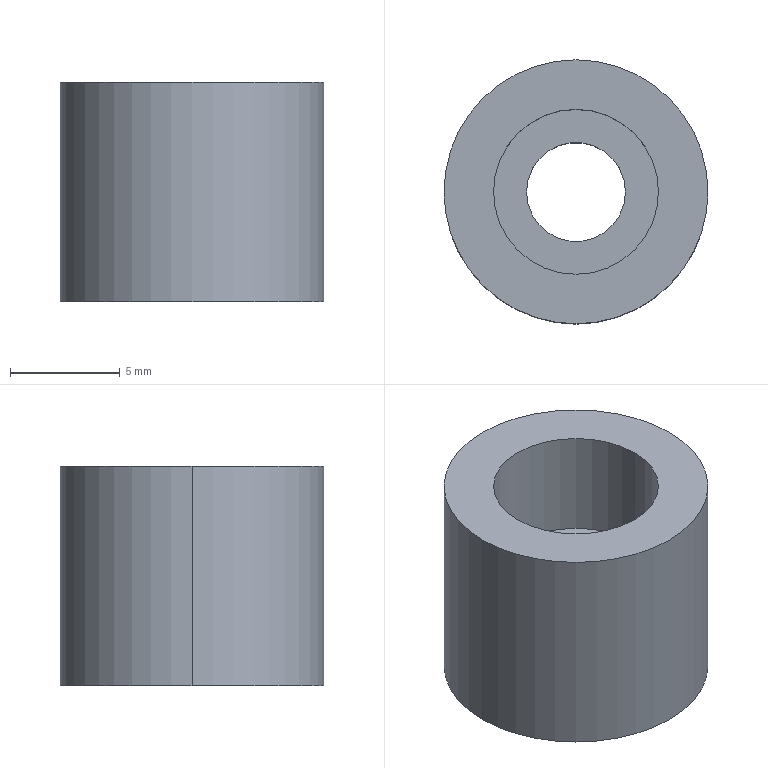Part | SolidWorks | features Extrusion 1, HoleWzd 1 | 1 solid | 9 faces | box 12 x 12 x 10 mm | volume 830.559 mm3 | cylinder 6 | plane 3 | commonest cylinder face diameters 4.5 x2 7.5 x2 12 x2
STEP:
#1=CARTESIAN_POINT('',(-3.75,0.,5.));
#2=VERTEX_POINT('',#1);
#3=CARTESIAN_POINT('',(3.75,0.,5.));
#4=VERTEX_POINT('',#3);
#5=CARTESIAN_POINT('',(0.,0.,5.));
#6=DIRECTION('',(0.,0.,1.));
#7=DIRECTION('',(1.,0.,0.));
#8=AXIS2_PLACEMENT_3D('',#5,#6,#7);
#9=CIRCLE('',#8,3.75);
#10=EDGE_CURVE('',#2,#4,#9,.T.);
#11=ORIENTED_EDGE('',*,*,#10,.F.);
#12=CARTESIAN_POINT('',(-3.75,0.,10.));
#13=VERTEX_POINT('',#12);
#14=CARTESIAN_POINT('',(-3.75,0.,10.));
#15=DIRECTION('',(0.,0.,1.));
#16=VECTOR('',#15,1000.);
#17=LINE('',#14,#16);
#18=EDGE_CURVE('',#2,#13,#17,.T.);
#19=ORIENTED_EDGE('',*,*,#18,.T.);
#20=CARTESIAN_POINT('',(3.75,0.,10.));
#21=VERTEX_POINT('',#20);
#22=CARTESIAN_POINT('',(0.,0.,10.));
#23=DIRECTION('',(0.,0.,1.));
#24=DIRECTION('',(1.,0.,0.));
#25=AXIS2_PLACEMENT_3D('',#22,#23,#24);
#26=CIRCLE('',#25,3.75);
#27=EDGE_CURVE('',#13,#21,#26,.T.);
#28=ORIENTED_EDGE('',*,*,#27,.T.);
#29=CARTESIAN_POINT('',(3.75,0.,10.));
#30=DIRECTION('',(0.,0.,1.));
#31=VECTOR('',#30,1000.);
#32=LINE('',#29,#31);
#33=EDGE_CURVE('',#4,#21,#32,.T.);
#34=ORIENTED_EDGE('',*,*,#33,.F.);
#35=EDGE_LOOP('',(#11,#19,#28,#34));
#36=FACE_OUTER_BOUND('',#35,.T.);
#37=CARTESIAN_POINT('',(0.,0.,10.));
#38=DIRECTION('',(0.,0.,1.));
#39=DIRECTION('',(1.,0.,0.));
#40=AXIS2_PLACEMENT_3D('',#37,#38,#39);
#41=CYLINDRICAL_SURFACE('',#40,3.75);
#42=ADVANCED_FACE('',(#36),#41,.F.);
#43=CARTESIAN_POINT('',(-2.25,0.,0.));
#44=VERTEX_POINT('',#43);
#45=CARTESIAN_POINT('',(2.25,0.,0.));
#46=VERTEX_POINT('',#45);
#47=CARTESIAN_POINT('',(0.,0.,0.));
#48=DIRECTION('',(0.,0.,1.));
#49=DIRECTION('',(1.,0.,0.));
#50=AXIS2_PLACEMENT_3D('',#47,#48,#49);
#51=CIRCLE('',#50,2.25);
#52=EDGE_CURVE('',#44,#46,#51,.T.);
#53=ORIENTED_EDGE('',*,*,#52,.F.);
#54=CARTESIAN_POINT('',(-2.25,0.,5.));
#55=VERTEX_POINT('',#54);
#56=CARTESIAN_POINT('',(-2.25,0.,10.));
#57=DIRECTION('',(0.,0.,1.));
#58=VECTOR('',#57,1000.);
#59=LINE('',#56,#58);
#60=EDGE_CURVE('',#44,#55,#59,.T.);
#61=ORIENTED_EDGE('',*,*,#60,.T.);
#62=CARTESIAN_POINT('',(2.25,0.,5.));
#63=VERTEX_POINT('',#62);
#64=CARTESIAN_POINT('',(0.,0.,5.));
#65=DIRECTION('',(0.,0.,1.));
#66=DIRECTION('',(1.,0.,0.));
#67=AXIS2_PLACEMENT_3D('',#64,#65,#66);
#68=CIRCLE('',#67,2.25);
#69=EDGE_CURVE('',#55,#63,#68,.T.);
#70=ORIENTED_EDGE('',*,*,#69,.T.);
#71=CARTESIAN_POINT('',(2.25,0.,10.));
#72=DIRECTION('',(0.,0.,1.));
#73=VECTOR('',#72,1000.);
#74=LINE('',#71,#73);
#75=EDGE_CURVE('',#46,#63,#74,.T.);
#76=ORIENTED_EDGE('',*,*,#75,.F.);
#77=EDGE_LOOP('',(#53,#61,#70,#76));
#78=FACE_OUTER_BOUND('',#77,.T.);
#79=CARTESIAN_POINT('',(0.,0.,10.));
#80=DIRECTION('',(0.,0.,1.));
#81=DIRECTION('',(1.,0.,0.));
#82=AXIS2_PLACEMENT_3D('',#79,#80,#81);
#83=CYLINDRICAL_SURFACE('',#82,2.25);
#84=ADVANCED_FACE('',(#78),#83,.F.);
#85=CARTESIAN_POINT('',(6.,0.,10.));
#86=VERTEX_POINT('',#85);
#87=CARTESIAN_POINT('',(-6.,0.,10.));
#88=VERTEX_POINT('',#87);
#89=CARTESIAN_POINT('',(0.,0.,10.));
#90=DIRECTION('',(0.,0.,1.));
#91=DIRECTION('',(1.,0.,0.));
#92=AXIS2_PLACEMENT_3D('',#89,#90,#91);
#93=CIRCLE('',#92,6.);
#94=EDGE_CURVE('',#86,#88,#93,.T.);
#95=ORIENTED_EDGE('',*,*,#94,.F.);
#96=CARTESIAN_POINT('',(6.,0.,0.));
#97=VERTEX_POINT('',#96);
#98=CARTESIAN_POINT('',(6.,0.,10.));
#99=DIRECTION('',(0.,0.,-1.));
#100=VECTOR('',#99,1000.);
#101=LINE('',#98,#100);
#102=EDGE_CURVE('',#86,#97,#101,.T.);
#103=ORIENTED_EDGE('',*,*,#102,.T.);
#104=CARTESIAN_POINT('',(-6.,0.,0.));
#105=VERTEX_POINT('',#104);
#106=CARTESIAN_POINT('',(0.,0.,0.));
#107=DIRECTION('',(0.,0.,1.));
#108=DIRECTION('',(1.,0.,0.));
#109=AXIS2_PLACEMENT_3D('',#106,#107,#108);
#110=CIRCLE('',#109,6.);
#111=EDGE_CURVE('',#97,#105,#110,.T.);
#112=ORIENTED_EDGE('',*,*,#111,.T.);
#113=CARTESIAN_POINT('',(-6.,0.,10.));
#114=DIRECTION('',(0.,0.,-1.));
#115=VECTOR('',#114,1000.);
#116=LINE('',#113,#115);
#117=EDGE_CURVE('',#88,#105,#116,.T.);
#118=ORIENTED_EDGE('',*,*,#117,.F.);
#119=EDGE_LOOP('',(#95,#103,#112,#118));
#120=FACE_OUTER_BOUND('',#119,.T.);
#121=CARTESIAN_POINT('',(0.,0.,10.));
#122=DIRECTION('',(0.,0.,-1.));
#123=DIRECTION('',(-1.,0.,0.));
#124=AXIS2_PLACEMENT_3D('',#121,#122,#123);
#125=CYLINDRICAL_SURFACE('',#124,6.);
#126=ADVANCED_FACE('',(#120),#125,.T.);
#127=ORIENTED_EDGE('',*,*,#102,.F.);
#128=CARTESIAN_POINT('',(0.,0.,10.));
#129=DIRECTION('',(0.,0.,1.));
#130=DIRECTION('',(1.,0.,0.));
#131=AXIS2_PLACEMENT_3D('',#128,#129,#130);
#132=CIRCLE('',#131,6.);
#133=EDGE_CURVE('',#88,#86,#132,.T.);
#134=ORIENTED_EDGE('',*,*,#133,.F.);
#135=ORIENTED_EDGE('',*,*,#117,.T.);
#136=CARTESIAN_POINT('',(0.,0.,0.));
#137=DIRECTION('',(0.,0.,1.));
#138=DIRECTION('',(1.,0.,0.));
#139=AXIS2_PLACEMENT_3D('',#136,#137,#138);
#140=CIRCLE('',#139,6.);
#141=EDGE_CURVE('',#105,#97,#140,.T.);
#142=ORIENTED_EDGE('',*,*,#141,.T.);
#143=EDGE_LOOP('',(#127,#134,#135,#142));
#144=FACE_OUTER_BOUND('',#143,.T.);
#145=CARTESIAN_POINT('',(0.,0.,10.));
#146=DIRECTION('',(0.,0.,-1.));
#147=DIRECTION('',(-1.,0.,0.));
#148=AXIS2_PLACEMENT_3D('',#145,#146,#147);
#149=CYLINDRICAL_SURFACE('',#148,6.);
#150=ADVANCED_FACE('',(#144),#149,.T.);
#151=CARTESIAN_POINT('',(0.,0.,10.));
#152=DIRECTION('',(0.,0.,1.));
#153=DIRECTION('',(1.,0.,0.));
#154=AXIS2_PLACEMENT_3D('',#151,#152,#153);
#155=CIRCLE('',#154,3.75);
#156=EDGE_CURVE('',#21,#13,#155,.T.);
#157=ORIENTED_EDGE('',*,*,#156,.F.);
#158=ORIENTED_EDGE('',*,*,#27,.F.);
#159=EDGE_LOOP('',(#157,#158));
#160=FACE_BOUND('',#159,.T.);
#161=ORIENTED_EDGE('',*,*,#133,.T.);
#162=ORIENTED_EDGE('',*,*,#94,.T.);
#163=EDGE_LOOP('',(#161,#162));
#164=FACE_OUTER_BOUND('',#163,.T.);
#165=CARTESIAN_POINT('',(0.,0.,10.));
#166=DIRECTION('',(0.,0.,1.));
#167=DIRECTION('',(1.,0.,0.));
#168=AXIS2_PLACEMENT_3D('',#165,#166,#167);
#169=PLANE('',#168);
#170=ADVANCED_FACE('',(#160,#164),#169,.T.);
#171=CARTESIAN_POINT('',(0.,0.,0.));
#172=DIRECTION('',(0.,0.,1.));
#173=DIRECTION('',(1.,0.,0.));
#174=AXIS2_PLACEMENT_3D('',#171,#172,#173);
#175=CIRCLE('',#174,2.25);
#176=EDGE_CURVE('',#46,#44,#175,.T.);
#177=ORIENTED_EDGE('',*,*,#176,.T.);
#178=ORIENTED_EDGE('',*,*,#52,.T.);
#179=EDGE_LOOP('',(#177,#178));
#180=FACE_BOUND('',#179,.T.);
#181=ORIENTED_EDGE('',*,*,#141,.F.);
#182=ORIENTED_EDGE('',*,*,#111,.F.);
#183=EDGE_LOOP('',(#181,#182));
#184=FACE_OUTER_BOUND('',#183,.T.);
#185=CARTESIAN_POINT('',(0.,0.,0.));
#186=DIRECTION('',(0.,0.,1.));
#187=DIRECTION('',(1.,0.,0.));
#188=AXIS2_PLACEMENT_3D('',#185,#186,#187);
#189=PLANE('',#188);
#190=ADVANCED_FACE('',(#180,#184),#189,.F.);
#191=ORIENTED_EDGE('',*,*,#60,.F.);
#192=ORIENTED_EDGE('',*,*,#176,.F.);
#193=ORIENTED_EDGE('',*,*,#75,.T.);
#194=CARTESIAN_POINT('',(0.,0.,5.));
#195=DIRECTION('',(0.,0.,1.));
#196=DIRECTION('',(1.,0.,0.));
#197=AXIS2_PLACEMENT_3D('',#194,#195,#196);
#198=CIRCLE('',#197,2.25);
#199=EDGE_CURVE('',#63,#55,#198,.T.);
#200=ORIENTED_EDGE('',*,*,#199,.T.);
#201=EDGE_LOOP('',(#191,#192,#193,#200));
#202=FACE_OUTER_BOUND('',#201,.T.);
#203=CARTESIAN_POINT('',(0.,0.,10.));
#204=DIRECTION('',(0.,0.,1.));
#205=DIRECTION('',(1.,0.,0.));
#206=AXIS2_PLACEMENT_3D('',#203,#204,#205);
#207=CYLINDRICAL_SURFACE('',#206,2.25);
#208=ADVANCED_FACE('',(#202),#207,.F.);
#209=ORIENTED_EDGE('',*,*,#199,.F.);
#210=ORIENTED_EDGE('',*,*,#69,.F.);
#211=EDGE_LOOP('',(#209,#210));
#212=FACE_BOUND('',#211,.T.);
#213=CARTESIAN_POINT('',(0.,0.,5.));
#214=DIRECTION('',(0.,0.,1.));
#215=DIRECTION('',(1.,0.,0.));
#216=AXIS2_PLACEMENT_3D('',#213,#214,#215);
#217=CIRCLE('',#216,3.75);
#218=EDGE_CURVE('',#4,#2,#217,.T.);
#219=ORIENTED_EDGE('',*,*,#218,.T.);
#220=ORIENTED_EDGE('',*,*,#10,.T.);
#221=EDGE_LOOP('',(#219,#220));
#222=FACE_OUTER_BOUND('',#221,.T.);
#223=CARTESIAN_POINT('',(2.25,0.,5.));
#224=DIRECTION('',(0.,0.,-1.));
#225=DIRECTION('',(-1.,0.,0.));
#226=AXIS2_PLACEMENT_3D('',#223,#224,#225);
#227=PLANE('',#226);
#228=ADVANCED_FACE('',(#212,#222),#227,.F.);
#229=ORIENTED_EDGE('',*,*,#18,.F.);
#230=ORIENTED_EDGE('',*,*,#218,.F.);
#231=ORIENTED_EDGE('',*,*,#33,.T.);
#232=ORIENTED_EDGE('',*,*,#156,.T.);
#233=EDGE_LOOP('',(#229,#230,#231,#232));
#234=FACE_OUTER_BOUND('',#233,.T.);
#235=CARTESIAN_POINT('',(0.,0.,10.));
#236=DIRECTION('',(0.,0.,1.));
#237=DIRECTION('',(1.,0.,0.));
#238=AXIS2_PLACEMENT_3D('',#235,#236,#237);
#239=CYLINDRICAL_SURFACE('',#238,3.75);
#240=ADVANCED_FACE('',(#234),#239,.F.);
#241=CLOSED_SHELL('',(#42,#84,#126,#150,#170,#190,#208,#228,#240));
#242=MANIFOLD_SOLID_BREP('',#241);
#243=CARTESIAN_POINT('',(0.,0.,0.));
#244=DIRECTION('',(0.,0.,1.));
#245=DIRECTION('',(1.,0.,0.));
#246=AXIS2_PLACEMENT_3D('',#243,#244,#245);
#247=(LENGTH_UNIT()NAMED_UNIT(*)SI_UNIT(.MILLI.,.METRE.));
#248=UNCERTAINTY_MEASURE_WITH_UNIT(LENGTH_MEASURE(0.00001),#247,'','');
#249=(NAMED_UNIT(*)PLANE_ANGLE_UNIT()SI_UNIT($,.RADIAN.));
#250=(NAMED_UNIT(*)SI_UNIT($,.STERADIAN.)SOLID_ANGLE_UNIT());
#251=(GEOMETRIC_REPRESENTATION_CONTEXT(3)GLOBAL_UNCERTAINTY_ASSIGNED_CONTEXT((#248))GLOBAL_UNIT_ASSIGNED_CONTEXT((#247,#249,#250))REPRESENTATION_CONTEXT('',''));
#252=ADVANCED_BREP_SHAPE_REPRESENTATION('',(#242,#246),#251);